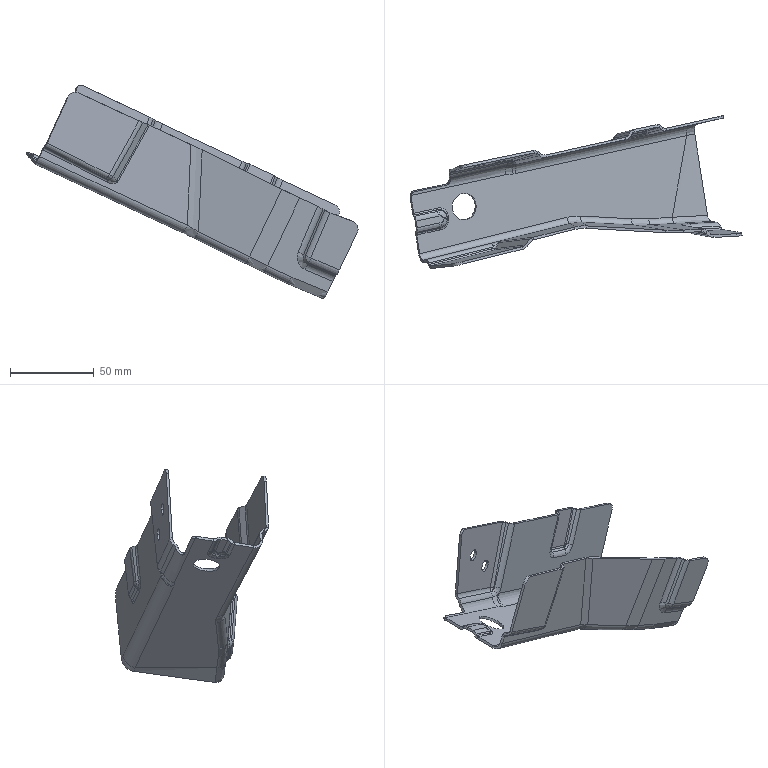Part | 1 solid | 243 faces | box 198.508 x 91.496 x 127.398 mm | volume 39999 mm3 | spline 157 | cylinder 58 | plane 19 | other 5 | sphere 2 | torus 2 | commonest cylinder face diameters 6 x12 10 x12 3 x9 7 x9 13 x4 9 x3